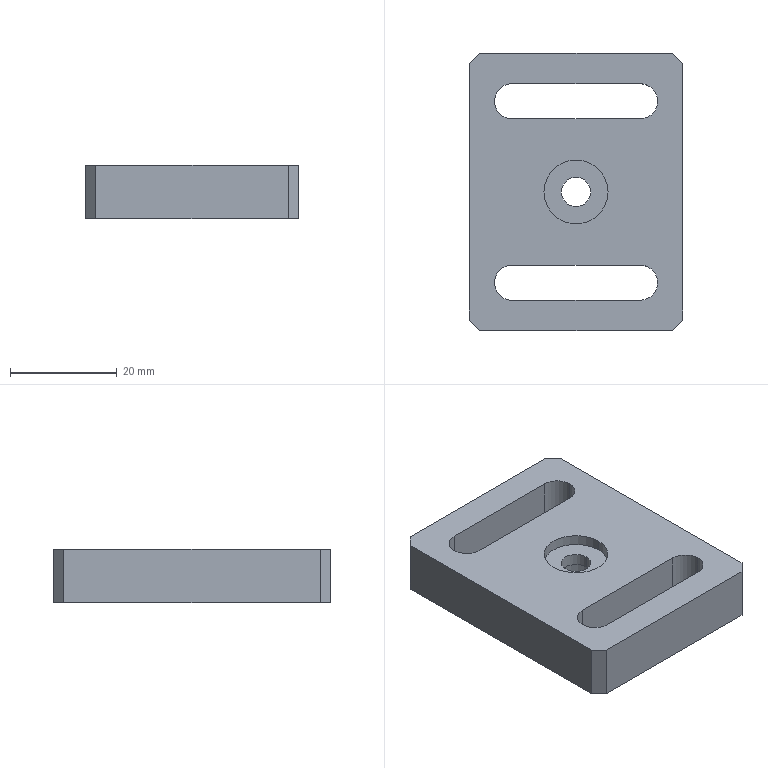Part | STEP file | 11-SMQ-00111 | 1 solid | 28 faces | box 40 x 52 x 10 mm | volume 16139 mm3 | plane 16 | cylinder 12 | commonest cylinder face diameters 6.6 x6 5.5 x2 10 x2 12 x2
STEP:
#1=CARTESIAN_POINT('',(15.3,-17.,0.));
#2=VERTEX_POINT('',#1);
#3=CARTESIAN_POINT('',(12.,-13.7,0.));
#4=VERTEX_POINT('',#3);
#5=CARTESIAN_POINT('',(12.,-17.,0.));
#6=DIRECTION('',(0.,0.,1.));
#7=DIRECTION('',(1.,0.,0.));
#8=AXIS2_PLACEMENT_3D('',#5,#6,#7);
#9=CIRCLE('',#8,3.3);
#10=EDGE_CURVE('',#2,#4,#9,.T.);
#11=ORIENTED_EDGE('',*,*,#10,.F.);
#12=CARTESIAN_POINT('',(15.3,-17.,10.));
#13=VERTEX_POINT('',#12);
#14=CARTESIAN_POINT('',(15.3,-17.,0.));
#15=DIRECTION('',(0.,0.,1.));
#16=VECTOR('',#15,1000.);
#17=LINE('',#14,#16);
#18=EDGE_CURVE('',#2,#13,#17,.T.);
#19=ORIENTED_EDGE('',*,*,#18,.T.);
#20=CARTESIAN_POINT('',(12.,-13.7,10.));
#21=VERTEX_POINT('',#20);
#22=CARTESIAN_POINT('',(12.,-17.,10.));
#23=DIRECTION('',(0.,0.,1.));
#24=DIRECTION('',(1.,0.,0.));
#25=AXIS2_PLACEMENT_3D('',#22,#23,#24);
#26=CIRCLE('',#25,3.3);
#27=EDGE_CURVE('',#13,#21,#26,.T.);
#28=ORIENTED_EDGE('',*,*,#27,.T.);
#29=CARTESIAN_POINT('',(12.,-13.7,0.));
#30=DIRECTION('',(0.,0.,1.));
#31=VECTOR('',#30,1000.);
#32=LINE('',#29,#31);
#33=EDGE_CURVE('',#4,#21,#32,.T.);
#34=ORIENTED_EDGE('',*,*,#33,.F.);
#35=EDGE_LOOP('',(#11,#19,#28,#34));
#36=FACE_OUTER_BOUND('',#35,.T.);
#37=CARTESIAN_POINT('',(12.,-17.,0.));
#38=DIRECTION('',(0.,0.,1.));
#39=DIRECTION('',(1.,0.,0.));
#40=AXIS2_PLACEMENT_3D('',#37,#38,#39);
#41=CYLINDRICAL_SURFACE('',#40,3.3);
#42=ADVANCED_FACE('',(#36),#41,.F.);
#43=CARTESIAN_POINT('',(15.3,17.,0.));
#44=VERTEX_POINT('',#43);
#45=CARTESIAN_POINT('',(12.,20.3,0.));
#46=VERTEX_POINT('',#45);
#47=CARTESIAN_POINT('',(12.,17.,0.));
#48=DIRECTION('',(0.,0.,1.));
#49=DIRECTION('',(1.,0.,0.));
#50=AXIS2_PLACEMENT_3D('',#47,#48,#49);
#51=CIRCLE('',#50,3.3);
#52=EDGE_CURVE('',#44,#46,#51,.T.);
#53=ORIENTED_EDGE('',*,*,#52,.F.);
#54=CARTESIAN_POINT('',(15.3,17.,10.));
#55=VERTEX_POINT('',#54);
#56=CARTESIAN_POINT('',(15.3,17.,0.));
#57=DIRECTION('',(0.,0.,1.));
#58=VECTOR('',#57,1000.);
#59=LINE('',#56,#58);
#60=EDGE_CURVE('',#44,#55,#59,.T.);
#61=ORIENTED_EDGE('',*,*,#60,.T.);
#62=CARTESIAN_POINT('',(12.,20.3,10.));
#63=VERTEX_POINT('',#62);
#64=CARTESIAN_POINT('',(12.,17.,10.));
#65=DIRECTION('',(0.,0.,1.));
#66=DIRECTION('',(1.,0.,0.));
#67=AXIS2_PLACEMENT_3D('',#64,#65,#66);
#68=CIRCLE('',#67,3.3);
#69=EDGE_CURVE('',#55,#63,#68,.T.);
#70=ORIENTED_EDGE('',*,*,#69,.T.);
#71=CARTESIAN_POINT('',(12.,20.3,0.));
#72=DIRECTION('',(0.,0.,1.));
#73=VECTOR('',#72,1000.);
#74=LINE('',#71,#73);
#75=EDGE_CURVE('',#46,#63,#74,.T.);
#76=ORIENTED_EDGE('',*,*,#75,.F.);
#77=EDGE_LOOP('',(#53,#61,#70,#76));
#78=FACE_OUTER_BOUND('',#77,.T.);
#79=CARTESIAN_POINT('',(12.,17.,0.));
#80=DIRECTION('',(0.,0.,1.));
#81=DIRECTION('',(1.,0.,0.));
#82=AXIS2_PLACEMENT_3D('',#79,#80,#81);
#83=CYLINDRICAL_SURFACE('',#82,3.3);
#84=ADVANCED_FACE('',(#78),#83,.F.);
#85=CARTESIAN_POINT('',(5.,0.,5.7));
#86=VERTEX_POINT('',#85);
#87=CARTESIAN_POINT('',(-5.,0.,5.7));
#88=VERTEX_POINT('',#87);
#89=CARTESIAN_POINT('',(0.,0.,5.7));
#90=DIRECTION('',(0.,0.,-1.));
#91=DIRECTION('',(-1.,0.,0.));
#92=AXIS2_PLACEMENT_3D('',#89,#90,#91);
#93=CIRCLE('',#92,5.);
#94=EDGE_CURVE('',#86,#88,#93,.T.);
#95=ORIENTED_EDGE('',*,*,#94,.F.);
#96=CARTESIAN_POINT('',(5.,0.,0.));
#97=VERTEX_POINT('',#96);
#98=CARTESIAN_POINT('',(5.,0.,0.));
#99=DIRECTION('',(0.,0.,-1.));
#100=VECTOR('',#99,1000.);
#101=LINE('',#98,#100);
#102=EDGE_CURVE('',#86,#97,#101,.T.);
#103=ORIENTED_EDGE('',*,*,#102,.T.);
#104=CARTESIAN_POINT('',(-5.,0.,0.));
#105=VERTEX_POINT('',#104);
#106=CARTESIAN_POINT('',(0.,0.,0.));
#107=DIRECTION('',(0.,0.,-1.));
#108=DIRECTION('',(-1.,0.,0.));
#109=AXIS2_PLACEMENT_3D('',#106,#107,#108);
#110=CIRCLE('',#109,5.);
#111=EDGE_CURVE('',#97,#105,#110,.T.);
#112=ORIENTED_EDGE('',*,*,#111,.T.);
#113=CARTESIAN_POINT('',(-5.,0.,0.));
#114=DIRECTION('',(0.,0.,-1.));
#115=VECTOR('',#114,1000.);
#116=LINE('',#113,#115);
#117=EDGE_CURVE('',#88,#105,#116,.T.);
#118=ORIENTED_EDGE('',*,*,#117,.F.);
#119=EDGE_LOOP('',(#95,#103,#112,#118));
#120=FACE_OUTER_BOUND('',#119,.T.);
#121=CARTESIAN_POINT('',(0.,0.,0.));
#122=DIRECTION('',(0.,0.,-1.));
#123=DIRECTION('',(-1.,0.,0.));
#124=AXIS2_PLACEMENT_3D('',#121,#122,#123);
#125=CYLINDRICAL_SURFACE('',#124,5.);
#126=ADVANCED_FACE('',(#120),#125,.F.);
#127=CARTESIAN_POINT('',(-2.75,0.,8.));
#128=VERTEX_POINT('',#127);
#129=CARTESIAN_POINT('',(2.75,0.,8.));
#130=VERTEX_POINT('',#129);
#131=CARTESIAN_POINT('',(0.,0.,8.));
#132=DIRECTION('',(0.,0.,1.));
#133=DIRECTION('',(1.,0.,0.));
#134=AXIS2_PLACEMENT_3D('',#131,#132,#133);
#135=CIRCLE('',#134,2.75);
#136=EDGE_CURVE('',#128,#130,#135,.T.);
#137=ORIENTED_EDGE('',*,*,#136,.T.);
#138=CARTESIAN_POINT('',(2.75,0.,5.7));
#139=VERTEX_POINT('',#138);
#140=CARTESIAN_POINT('',(2.75,0.,0.));
#141=DIRECTION('',(0.,0.,-1.));
#142=VECTOR('',#141,1000.);
#143=LINE('',#140,#142);
#144=EDGE_CURVE('',#130,#139,#143,.T.);
#145=ORIENTED_EDGE('',*,*,#144,.T.);
#146=CARTESIAN_POINT('',(-2.75,0.,5.7));
#147=VERTEX_POINT('',#146);
#148=CARTESIAN_POINT('',(0.,0.,5.7));
#149=DIRECTION('',(0.,0.,-1.));
#150=DIRECTION('',(-1.,0.,0.));
#151=AXIS2_PLACEMENT_3D('',#148,#149,#150);
#152=CIRCLE('',#151,2.75);
#153=EDGE_CURVE('',#139,#147,#152,.T.);
#154=ORIENTED_EDGE('',*,*,#153,.T.);
#155=CARTESIAN_POINT('',(-2.75,0.,0.));
#156=DIRECTION('',(0.,0.,-1.));
#157=VECTOR('',#156,1000.);
#158=LINE('',#155,#157);
#159=EDGE_CURVE('',#128,#147,#158,.T.);
#160=ORIENTED_EDGE('',*,*,#159,.F.);
#161=EDGE_LOOP('',(#137,#145,#154,#160));
#162=FACE_OUTER_BOUND('',#161,.T.);
#163=CARTESIAN_POINT('',(0.,0.,0.));
#164=DIRECTION('',(0.,0.,-1.));
#165=DIRECTION('',(-1.,0.,0.));
#166=AXIS2_PLACEMENT_3D('',#163,#164,#165);
#167=CYLINDRICAL_SURFACE('',#166,2.75);
#168=ADVANCED_FACE('',(#162),#167,.F.);
#169=CARTESIAN_POINT('',(-6.,0.,8.));
#170=VERTEX_POINT('',#169);
#171=CARTESIAN_POINT('',(6.,0.,8.));
#172=VERTEX_POINT('',#171);
#173=CARTESIAN_POINT('',(0.,0.,8.));
#174=DIRECTION('',(0.,0.,1.));
#175=DIRECTION('',(1.,0.,0.));
#176=AXIS2_PLACEMENT_3D('',#173,#174,#175);
#177=CIRCLE('',#176,6.);
#178=EDGE_CURVE('',#170,#172,#177,.T.);
#179=ORIENTED_EDGE('',*,*,#178,.F.);
#180=CARTESIAN_POINT('',(-6.,0.,10.));
#181=VERTEX_POINT('',#180);
#182=CARTESIAN_POINT('',(-6.,0.,8.));
#183=DIRECTION('',(0.,0.,1.));
#184=VECTOR('',#183,1000.);
#185=LINE('',#182,#184);
#186=EDGE_CURVE('',#170,#181,#185,.T.);
#187=ORIENTED_EDGE('',*,*,#186,.T.);
#188=CARTESIAN_POINT('',(6.,0.,10.));
#189=VERTEX_POINT('',#188);
#190=CARTESIAN_POINT('',(0.,0.,10.));
#191=DIRECTION('',(0.,0.,1.));
#192=DIRECTION('',(1.,0.,0.));
#193=AXIS2_PLACEMENT_3D('',#190,#191,#192);
#194=CIRCLE('',#193,6.);
#195=EDGE_CURVE('',#181,#189,#194,.T.);
#196=ORIENTED_EDGE('',*,*,#195,.T.);
#197=CARTESIAN_POINT('',(6.,0.,8.));
#198=DIRECTION('',(0.,0.,1.));
#199=VECTOR('',#198,1000.);
#200=LINE('',#197,#199);
#201=EDGE_CURVE('',#172,#189,#200,.T.);
#202=ORIENTED_EDGE('',*,*,#201,.F.);
#203=EDGE_LOOP('',(#179,#187,#196,#202));
#204=FACE_OUTER_BOUND('',#203,.T.);
#205=CARTESIAN_POINT('',(0.,0.,8.));
#206=DIRECTION('',(0.,0.,1.));
#207=DIRECTION('',(1.,0.,0.));
#208=AXIS2_PLACEMENT_3D('',#205,#206,#207);
#209=CYLINDRICAL_SURFACE('',#208,6.);
#210=ADVANCED_FACE('',(#204),#209,.F.);
#211=CARTESIAN_POINT('',(20.,-24.,10.));
#212=VERTEX_POINT('',#211);
#213=CARTESIAN_POINT('',(20.,24.,10.));
#214=VERTEX_POINT('',#213);
#215=CARTESIAN_POINT('',(20.,-26.,10.));
#216=DIRECTION('',(0.,1.,0.));
#217=VECTOR('',#216,1000.);
#218=LINE('',#215,#217);
#219=EDGE_CURVE('',#212,#214,#218,.T.);
#220=ORIENTED_EDGE('',*,*,#219,.F.);
#221=CARTESIAN_POINT('',(20.,-24.,0.));
#222=VERTEX_POINT('',#221);
#223=CARTESIAN_POINT('',(20.,-24.,10.));
#224=DIRECTION('',(0.,0.,-1.));
#225=VECTOR('',#224,1000.);
#226=LINE('',#223,#225);
#227=EDGE_CURVE('',#212,#222,#226,.T.);
#228=ORIENTED_EDGE('',*,*,#227,.T.);
#229=CARTESIAN_POINT('',(20.,24.,0.));
#230=VERTEX_POINT('',#229);
#231=CARTESIAN_POINT('',(20.,-26.,0.));
#232=DIRECTION('',(0.,1.,0.));
#233=VECTOR('',#232,1000.);
#234=LINE('',#231,#233);
#235=EDGE_CURVE('',#222,#230,#234,.T.);
#236=ORIENTED_EDGE('',*,*,#235,.T.);
#237=CARTESIAN_POINT('',(20.,24.,10.));
#238=DIRECTION('',(0.,0.,1.));
#239=VECTOR('',#238,1000.);
#240=LINE('',#237,#239);
#241=EDGE_CURVE('',#230,#214,#240,.T.);
#242=ORIENTED_EDGE('',*,*,#241,.T.);
#243=EDGE_LOOP('',(#220,#228,#236,#242));
#244=FACE_OUTER_BOUND('',#243,.T.);
#245=CARTESIAN_POINT('',(20.,-26.,10.));
#246=DIRECTION('',(-1.,0.,0.));
#247=DIRECTION('',(0.,0.,1.));
#248=AXIS2_PLACEMENT_3D('',#245,#246,#247);
#249=PLANE('',#248);
#250=ADVANCED_FACE('',(#244),#249,.F.);
#251=CARTESIAN_POINT('',(18.,26.,10.));
#252=VERTEX_POINT('',#251);
#253=CARTESIAN_POINT('',(-18.,26.,10.));
#254=VERTEX_POINT('',#253);
#255=CARTESIAN_POINT('',(-20.,26.,10.));
#256=DIRECTION('',(-1.,0.,0.));
#257=VECTOR('',#256,1000.);
#258=LINE('',#255,#257);
#259=EDGE_CURVE('',#252,#254,#258,.T.);
#260=ORIENTED_EDGE('',*,*,#259,.F.);
#261=CARTESIAN_POINT('',(18.,26.,0.));
#262=VERTEX_POINT('',#261);
#263=CARTESIAN_POINT('',(18.,26.,10.));
#264=DIRECTION('',(0.,0.,-1.));
#265=VECTOR('',#264,1000.);
#266=LINE('',#263,#265);
#267=EDGE_CURVE('',#252,#262,#266,.T.);
#268=ORIENTED_EDGE('',*,*,#267,.T.);
#269=CARTESIAN_POINT('',(-18.,26.,0.));
#270=VERTEX_POINT('',#269);
#271=CARTESIAN_POINT('',(-20.,26.,0.));
#272=DIRECTION('',(-1.,0.,0.));
#273=VECTOR('',#272,1000.);
#274=LINE('',#271,#273);
#275=EDGE_CURVE('',#262,#270,#274,.T.);
#276=ORIENTED_EDGE('',*,*,#275,.T.);
#277=CARTESIAN_POINT('',(-18.,26.,10.));
#278=DIRECTION('',(0.,0.,1.));
#279=VECTOR('',#278,1000.);
#280=LINE('',#277,#279);
#281=EDGE_CURVE('',#270,#254,#280,.T.);
#282=ORIENTED_EDGE('',*,*,#281,.T.);
#283=EDGE_LOOP('',(#260,#268,#276,#282));
#284=FACE_OUTER_BOUND('',#283,.T.);
#285=CARTESIAN_POINT('',(-20.,26.,10.));
#286=DIRECTION('',(0.,-1.,0.));
#287=DIRECTION('',(0.,0.,-1.));
#288=AXIS2_PLACEMENT_3D('',#285,#286,#287);
#289=PLANE('',#288);
#290=ADVANCED_FACE('',(#284),#289,.F.);
#291=CARTESIAN_POINT('',(-20.,24.,0.));
#292=VERTEX_POINT('',#291);
#293=CARTESIAN_POINT('',(-20.,-24.,0.));
#294=VERTEX_POINT('',#293);
#295=CARTESIAN_POINT('',(-20.,-26.,0.));
#296=DIRECTION('',(0.,-1.,0.));
#297=VECTOR('',#296,1000.);
#298=LINE('',#295,#297);
#299=EDGE_CURVE('',#292,#294,#298,.T.);
#300=ORIENTED_EDGE('',*,*,#299,.T.);
#301=CARTESIAN_POINT('',(-20.,-24.,10.));
#302=VERTEX_POINT('',#301);
#303=CARTESIAN_POINT('',(-20.,-24.,10.));
#304=DIRECTION('',(0.,0.,1.));
#305=VECTOR('',#304,1000.);
#306=LINE('',#303,#305);
#307=EDGE_CURVE('',#294,#302,#306,.T.);
#308=ORIENTED_EDGE('',*,*,#307,.T.);
#309=CARTESIAN_POINT('',(-20.,24.,10.));
#310=VERTEX_POINT('',#309);
#311=CARTESIAN_POINT('',(-20.,-26.,10.));
#312=DIRECTION('',(0.,-1.,0.));
#313=VECTOR('',#312,1000.);
#314=LINE('',#311,#313);
#315=EDGE_CURVE('',#310,#302,#314,.T.);
#316=ORIENTED_EDGE('',*,*,#315,.F.);
#317=CARTESIAN_POINT('',(-20.,24.,10.));
#318=DIRECTION('',(0.,0.,-1.));
#319=VECTOR('',#318,1000.);
#320=LINE('',#317,#319);
#321=EDGE_CURVE('',#310,#292,#320,.T.);
#322=ORIENTED_EDGE('',*,*,#321,.T.);
#323=EDGE_LOOP('',(#300,#308,#316,#322));
#324=FACE_OUTER_BOUND('',#323,.T.);
#325=CARTESIAN_POINT('',(-20.,-26.,10.));
#326=DIRECTION('',(1.,0.,0.));
#327=DIRECTION('',(0.,0.,-1.));
#328=AXIS2_PLACEMENT_3D('',#325,#326,#327);
#329=PLANE('',#328);
#330=ADVANCED_FACE('',(#324),#329,.F.);
#331=CARTESIAN_POINT('',(-18.,-26.,0.));
#332=VERTEX_POINT('',#331);
#333=CARTESIAN_POINT('',(18.,-26.,0.));
#334=VERTEX_POINT('',#333);
#335=CARTESIAN_POINT('',(-20.,-26.,0.));
#336=DIRECTION('',(1.,0.,0.));
#337=VECTOR('',#336,1000.);
#338=LINE('',#335,#337);
#339=EDGE_CURVE('',#332,#334,#338,.T.);
#340=ORIENTED_EDGE('',*,*,#339,.T.);
#341=CARTESIAN_POINT('',(18.,-26.,10.));
#342=VERTEX_POINT('',#341);
#343=CARTESIAN_POINT('',(18.,-26.,10.));
#344=DIRECTION('',(0.,0.,1.));
#345=VECTOR('',#344,1000.);
#346=LINE('',#343,#345);
#347=EDGE_CURVE('',#334,#342,#346,.T.);
#348=ORIENTED_EDGE('',*,*,#347,.T.);
#349=CARTESIAN_POINT('',(-18.,-26.,10.));
#350=VERTEX_POINT('',#349);
#351=CARTESIAN_POINT('',(-20.,-26.,10.));
#352=DIRECTION('',(1.,0.,0.));
#353=VECTOR('',#352,1000.);
#354=LINE('',#351,#353);
#355=EDGE_CURVE('',#350,#342,#354,.T.);
#356=ORIENTED_EDGE('',*,*,#355,.F.);
#357=CARTESIAN_POINT('',(-18.,-26.,10.));
#358=DIRECTION('',(0.,0.,-1.));
#359=VECTOR('',#358,1000.);
#360=LINE('',#357,#359);
#361=EDGE_CURVE('',#350,#332,#360,.T.);
#362=ORIENTED_EDGE('',*,*,#361,.T.);
#363=EDGE_LOOP('',(#340,#348,#356,#362));
#364=FACE_OUTER_BOUND('',#363,.T.);
#365=CARTESIAN_POINT('',(-20.,-26.,10.));
#366=DIRECTION('',(0.,1.,0.));
#367=DIRECTION('',(0.,0.,1.));
#368=AXIS2_PLACEMENT_3D('',#365,#366,#367);
#369=PLANE('',#368);
#370=ADVANCED_FACE('',(#364),#369,.F.);
#371=CARTESIAN_POINT('',(-12.,-13.7,10.));
#372=VERTEX_POINT('',#371);
#373=CARTESIAN_POINT('',(12.,-13.7,10.));
#374=DIRECTION('',(-1.,0.,0.));
#375=VECTOR('',#374,1000.);
#376=LINE('',#373,#375);
#377=EDGE_CURVE('',#21,#372,#376,.T.);
#378=ORIENTED_EDGE('',*,*,#377,.F.);
#379=ORIENTED_EDGE('',*,*,#27,.F.);
#380=CARTESIAN_POINT('',(12.,-20.3,10.));
#381=VERTEX_POINT('',#380);
#382=CARTESIAN_POINT('',(12.,-17.,10.));
#383=DIRECTION('',(0.,0.,1.));
#384=DIRECTION('',(1.,0.,0.));
#385=AXIS2_PLACEMENT_3D('',#382,#383,#384);
#386=CIRCLE('',#385,3.3);
#387=EDGE_CURVE('',#381,#13,#386,.T.);
#388=ORIENTED_EDGE('',*,*,#387,.F.);
#389=CARTESIAN_POINT('',(-12.,-20.3,10.));
#390=VERTEX_POINT('',#389);
#391=CARTESIAN_POINT('',(12.,-20.3,10.));
#392=DIRECTION('',(1.,0.,0.));
#393=VECTOR('',#392,1000.);
#394=LINE('',#391,#393);
#395=EDGE_CURVE('',#390,#381,#394,.T.);
#396=ORIENTED_EDGE('',*,*,#395,.F.);
#397=CARTESIAN_POINT('',(-12.,-17.,10.));
#398=DIRECTION('',(0.,0.,1.));
#399=DIRECTION('',(1.,0.,0.));
#400=AXIS2_PLACEMENT_3D('',#397,#398,#399);
#401=CIRCLE('',#400,3.3);
#402=EDGE_CURVE('',#372,#390,#401,.T.);
#403=ORIENTED_EDGE('',*,*,#402,.F.);
#404=EDGE_LOOP('',(#378,#379,#388,#396,#403));
#405=FACE_BOUND('',#404,.T.);
#406=CARTESIAN_POINT('',(-12.,20.3,10.));
#407=VERTEX_POINT('',#406);
#408=CARTESIAN_POINT('',(12.,20.3,10.));
#409=DIRECTION('',(-1.,0.,0.));
#410=VECTOR('',#409,1000.);
#411=LINE('',#408,#410);
#412=EDGE_CURVE('',#63,#407,#411,.T.);
#413=ORIENTED_EDGE('',*,*,#412,.F.);
#414=ORIENTED_EDGE('',*,*,#69,.F.);
#415=CARTESIAN_POINT('',(12.,13.7,10.));
#416=VERTEX_POINT('',#415);
#417=CARTESIAN_POINT('',(12.,17.,10.));
#418=DIRECTION('',(0.,0.,1.));
#419=DIRECTION('',(1.,0.,0.));
#420=AXIS2_PLACEMENT_3D('',#417,#418,#419);
#421=CIRCLE('',#420,3.3);
#422=EDGE_CURVE('',#416,#55,#421,.T.);
#423=ORIENTED_EDGE('',*,*,#422,.F.);
#424=CARTESIAN_POINT('',(-12.,13.7,10.));
#425=VERTEX_POINT('',#424);
#426=CARTESIAN_POINT('',(12.,13.7,10.));
#427=DIRECTION('',(1.,0.,0.));
#428=VECTOR('',#427,1000.);
#429=LINE('',#426,#428);
#430=EDGE_CURVE('',#425,#416,#429,.T.);
#431=ORIENTED_EDGE('',*,*,#430,.F.);
#432=CARTESIAN_POINT('',(-12.,17.,10.));
#433=DIRECTION('',(0.,0.,1.));
#434=DIRECTION('',(1.,0.,0.));
#435=AXIS2_PLACEMENT_3D('',#432,#433,#434);
#436=CIRCLE('',#435,3.3);
#437=EDGE_CURVE('',#407,#425,#436,.T.);
#438=ORIENTED_EDGE('',*,*,#437,.F.);
#439=EDGE_LOOP('',(#413,#414,#423,#431,#438));
#440=FACE_BOUND('',#439,.T.);
#441=CARTESIAN_POINT('',(0.,0.,10.));
#442=DIRECTION('',(0.,0.,1.));
#443=DIRECTION('',(1.,0.,0.));
#444=AXIS2_PLACEMENT_3D('',#441,#442,#443);
#445=CIRCLE('',#444,6.);
#446=EDGE_CURVE('',#189,#181,#445,.T.);
#447=ORIENTED_EDGE('',*,*,#446,.F.);
#448=ORIENTED_EDGE('',*,*,#195,.F.);
#449=EDGE_LOOP('',(#447,#448));
#450=FACE_BOUND('',#449,.T.);
#451=ORIENTED_EDGE('',*,*,#355,.T.);
#452=CARTESIAN_POINT('',(20.,-24.,10.));
#453=DIRECTION('',(0.7071,0.7071,0.));
#454=VECTOR('',#453,1000.);
#455=LINE('',#452,#454);
#456=EDGE_CURVE('',#342,#212,#455,.T.);
#457=ORIENTED_EDGE('',*,*,#456,.T.);
#458=ORIENTED_EDGE('',*,*,#219,.T.);
#459=CARTESIAN_POINT('',(18.,26.,10.));
#460=DIRECTION('',(-0.7071,0.7071,0.));
#461=VECTOR('',#460,1000.);
#462=LINE('',#459,#461);
#463=EDGE_CURVE('',#214,#252,#462,.T.);
#464=ORIENTED_EDGE('',*,*,#463,.T.);
#465=ORIENTED_EDGE('',*,*,#259,.T.);
#466=CARTESIAN_POINT('',(-20.,24.,10.));
#467=DIRECTION('',(-0.7071,-0.7071,0.));
#468=VECTOR('',#467,1000.);
#469=LINE('',#466,#468);
#470=EDGE_CURVE('',#254,#310,#469,.T.);
#471=ORIENTED_EDGE('',*,*,#470,.T.);
#472=ORIENTED_EDGE('',*,*,#315,.T.);
#473=CARTESIAN_POINT('',(-18.,-26.,10.));
#474=DIRECTION('',(0.7071,-0.7071,0.));
#475=VECTOR('',#474,1000.);
#476=LINE('',#473,#475);
#477=EDGE_CURVE('',#302,#350,#476,.T.);
#478=ORIENTED_EDGE('',*,*,#477,.T.);
#479=EDGE_LOOP('',(#451,#457,#458,#464,#465,#471,#472,#478));
#480=FACE_OUTER_BOUND('',#479,.T.);
#481=CARTESIAN_POINT('',(0.,0.,10.));
#482=DIRECTION('',(0.,0.,-1.));
#483=DIRECTION('',(-1.,0.,0.));
#484=AXIS2_PLACEMENT_3D('',#481,#482,#483);
#485=PLANE('',#484);
#486=ADVANCED_FACE('',(#405,#440,#450,#480),#485,.F.);
#487=CARTESIAN_POINT('',(12.,-20.3,0.));
#488=VERTEX_POINT('',#487);
#489=CARTESIAN_POINT('',(12.,-17.,0.));
#490=DIRECTION('',(0.,0.,1.));
#491=DIRECTION('',(1.,0.,0.));
#492=AXIS2_PLACEMENT_3D('',#489,#490,#491);
#493=CIRCLE('',#492,3.3);
#494=EDGE_CURVE('',#488,#2,#493,.T.);
#495=ORIENTED_EDGE('',*,*,#494,.T.);
#496=ORIENTED_EDGE('',*,*,#10,.T.);
#497=CARTESIAN_POINT('',(-12.,-13.7,0.));
#498=VERTEX_POINT('',#497);
#499=CARTESIAN_POINT('',(12.,-13.7,0.));
#500=DIRECTION('',(-1.,0.,0.));
#501=VECTOR('',#500,1000.);
#502=LINE('',#499,#501);
#503=EDGE_CURVE('',#4,#498,#502,.T.);
#504=ORIENTED_EDGE('',*,*,#503,.T.);
#505=CARTESIAN_POINT('',(-12.,-20.3,0.));
#506=VERTEX_POINT('',#505);
#507=CARTESIAN_POINT('',(-12.,-17.,0.));
#508=DIRECTION('',(0.,0.,1.));
#509=DIRECTION('',(1.,0.,0.));
#510=AXIS2_PLACEMENT_3D('',#507,#508,#509);
#511=CIRCLE('',#510,3.3);
#512=EDGE_CURVE('',#498,#506,#511,.T.);
#513=ORIENTED_EDGE('',*,*,#512,.T.);
#514=CARTESIAN_POINT('',(12.,-20.3,0.));
#515=DIRECTION('',(1.,0.,0.));
#516=VECTOR('',#515,1000.);
#517=LINE('',#514,#516);
#518=EDGE_CURVE('',#506,#488,#517,.T.);
#519=ORIENTED_EDGE('',*,*,#518,.T.);
#520=EDGE_LOOP('',(#495,#496,#504,#513,#519));
#521=FACE_BOUND('',#520,.T.);
#522=CARTESIAN_POINT('',(12.,13.7,0.));
#523=VERTEX_POINT('',#522);
#524=CARTESIAN_POINT('',(12.,17.,0.));
#525=DIRECTION('',(0.,0.,1.));
#526=DIRECTION('',(1.,0.,0.));
#527=AXIS2_PLACEMENT_3D('',#524,#525,#526);
#528=CIRCLE('',#527,3.3);
#529=EDGE_CURVE('',#523,#44,#528,.T.);
#530=ORIENTED_EDGE('',*,*,#529,.T.);
#531=ORIENTED_EDGE('',*,*,#52,.T.);
#532=CARTESIAN_POINT('',(-12.,20.3,0.));
#533=VERTEX_POINT('',#532);
#534=CARTESIAN_POINT('',(12.,20.3,0.));
#535=DIRECTION('',(-1.,0.,0.));
#536=VECTOR('',#535,1000.);
#537=LINE('',#534,#536);
#538=EDGE_CURVE('',#46,#533,#537,.T.);
#539=ORIENTED_EDGE('',*,*,#538,.T.);
#540=CARTESIAN_POINT('',(-12.,13.7,0.));
#541=VERTEX_POINT('',#540);
#542=CARTESIAN_POINT('',(-12.,17.,0.));
#543=DIRECTION('',(0.,0.,1.));
#544=DIRECTION('',(1.,0.,0.));
#545=AXIS2_PLACEMENT_3D('',#542,#543,#544);
#546=CIRCLE('',#545,3.3);
#547=EDGE_CURVE('',#533,#541,#546,.T.);
#548=ORIENTED_EDGE('',*,*,#547,.T.);
#549=CARTESIAN_POINT('',(12.,13.7,0.));
#550=DIRECTION('',(1.,0.,0.));
#551=VECTOR('',#550,1000.);
#552=LINE('',#549,#551);
#553=EDGE_CURVE('',#541,#523,#552,.T.);
#554=ORIENTED_EDGE('',*,*,#553,.T.);
#555=EDGE_LOOP('',(#530,#531,#539,#548,#554));
#556=FACE_BOUND('',#555,.T.);
#557=CARTESIAN_POINT('',(0.,0.,0.));
#558=DIRECTION('',(0.,0.,-1.));
#559=DIRECTION('',(-1.,0.,0.));
#560=AXIS2_PLACEMENT_3D('',#557,#558,#559);
#561=CIRCLE('',#560,5.);
#562=EDGE_CURVE('',#105,#97,#561,.T.);
#563=ORIENTED_EDGE('',*,*,#562,.F.);
#564=ORIENTED_EDGE('',*,*,#111,.F.);
#565=EDGE_LOOP('',(#563,#564));
#566=FACE_BOUND('',#565,.T.);
#567=ORIENTED_EDGE('',*,*,#235,.F.);
#568=CARTESIAN_POINT('',(22.,-22.,0.));
#569=DIRECTION('',(-0.7071,-0.7071,0.));
#570=VECTOR('',#569,1000.);
#571=LINE('',#568,#570);
#572=EDGE_CURVE('',#222,#334,#571,.T.);
#573=ORIENTED_EDGE('',*,*,#572,.T.);
#574=ORIENTED_EDGE('',*,*,#339,.F.);
#575=CARTESIAN_POINT('',(-22.,-22.,0.));
#576=DIRECTION('',(-0.7071,0.7071,0.));
#577=VECTOR('',#576,1000.);
#578=LINE('',#575,#577);
#579=EDGE_CURVE('',#332,#294,#578,.T.);
#580=ORIENTED_EDGE('',*,*,#579,.T.);
#581=ORIENTED_EDGE('',*,*,#299,.F.);
#582=CARTESIAN_POINT('',(-22.,22.,0.));
#583=DIRECTION('',(0.7071,0.7071,0.));
#584=VECTOR('',#583,1000.);
#585=LINE('',#582,#584);
#586=EDGE_CURVE('',#292,#270,#585,.T.);
#587=ORIENTED_EDGE('',*,*,#586,.T.);
#588=ORIENTED_EDGE('',*,*,#275,.F.);
#589=CARTESIAN_POINT('',(22.,22.,0.));
#590=DIRECTION('',(0.7071,-0.7071,0.));
#591=VECTOR('',#590,1000.);
#592=LINE('',#589,#591);
#593=EDGE_CURVE('',#262,#230,#592,.T.);
#594=ORIENTED_EDGE('',*,*,#593,.T.);
#595=EDGE_LOOP('',(#567,#573,#574,#580,#581,#587,#588,#594));
#596=FACE_OUTER_BOUND('',#595,.T.);
#597=CARTESIAN_POINT('',(0.,0.,0.));
#598=DIRECTION('',(0.,0.,-1.));
#599=DIRECTION('',(-1.,0.,0.));
#600=AXIS2_PLACEMENT_3D('',#597,#598,#599);
#601=PLANE('',#600);
#602=ADVANCED_FACE('',(#521,#556,#566,#596),#601,.T.);
#603=ORIENTED_EDGE('',*,*,#456,.F.);
#604=ORIENTED_EDGE('',*,*,#347,.F.);
#605=ORIENTED_EDGE('',*,*,#572,.F.);
#606=ORIENTED_EDGE('',*,*,#227,.F.);
#607=EDGE_LOOP('',(#603,#604,#605,#606));
#608=FACE_OUTER_BOUND('',#607,.T.);
#609=CARTESIAN_POINT('',(20.,-24.,10.));
#610=DIRECTION('',(-0.7071,0.7071,0.));
#611=DIRECTION('',(0.,0.,-1.));
#612=AXIS2_PLACEMENT_3D('',#609,#610,#611);
#613=PLANE('',#612);
#614=ADVANCED_FACE('',(#608),#613,.F.);
#615=ORIENTED_EDGE('',*,*,#463,.F.);
#616=ORIENTED_EDGE('',*,*,#241,.F.);
#617=ORIENTED_EDGE('',*,*,#593,.F.);
#618=ORIENTED_EDGE('',*,*,#267,.F.);
#619=EDGE_LOOP('',(#615,#616,#617,#618));
#620=FACE_OUTER_BOUND('',#619,.T.);
#621=CARTESIAN_POINT('',(18.,26.,10.));
#622=DIRECTION('',(-0.7071,-0.7071,0.));
#623=DIRECTION('',(0.,0.,-1.));
#624=AXIS2_PLACEMENT_3D('',#621,#622,#623);
#625=PLANE('',#624);
#626=ADVANCED_FACE('',(#620),#625,.F.);
#627=ORIENTED_EDGE('',*,*,#477,.F.);
#628=ORIENTED_EDGE('',*,*,#307,.F.);
#629=ORIENTED_EDGE('',*,*,#579,.F.);
#630=ORIENTED_EDGE('',*,*,#361,.F.);
#631=EDGE_LOOP('',(#627,#628,#629,#630));
#632=FACE_OUTER_BOUND('',#631,.T.);
#633=CARTESIAN_POINT('',(-18.,-26.,10.));
#634=DIRECTION('',(0.7071,0.7071,0.));
#635=DIRECTION('',(0.,0.,-1.));
#636=AXIS2_PLACEMENT_3D('',#633,#634,#635);
#637=PLANE('',#636);
#638=ADVANCED_FACE('',(#632),#637,.F.);
#639=ORIENTED_EDGE('',*,*,#470,.F.);
#640=ORIENTED_EDGE('',*,*,#281,.F.);
#641=ORIENTED_EDGE('',*,*,#586,.F.);
#642=ORIENTED_EDGE('',*,*,#321,.F.);
#643=EDGE_LOOP('',(#639,#640,#641,#642));
#644=FACE_OUTER_BOUND('',#643,.T.);
#645=CARTESIAN_POINT('',(-20.,24.,10.));
#646=DIRECTION('',(0.7071,-0.7071,0.));
#647=DIRECTION('',(0.,0.,-1.));
#648=AXIS2_PLACEMENT_3D('',#645,#646,#647);
#649=PLANE('',#648);
#650=ADVANCED_FACE('',(#644),#649,.F.);
#651=ORIENTED_EDGE('',*,*,#186,.F.);
#652=CARTESIAN_POINT('',(0.,0.,8.));
#653=DIRECTION('',(0.,0.,1.));
#654=DIRECTION('',(1.,0.,0.));
#655=AXIS2_PLACEMENT_3D('',#652,#653,#654);
#656=CIRCLE('',#655,6.);
#657=EDGE_CURVE('',#172,#170,#656,.T.);
#658=ORIENTED_EDGE('',*,*,#657,.F.);
#659=ORIENTED_EDGE('',*,*,#201,.T.);
#660=ORIENTED_EDGE('',*,*,#446,.T.);
#661=EDGE_LOOP('',(#651,#658,#659,#660));
#662=FACE_OUTER_BOUND('',#661,.T.);
#663=CARTESIAN_POINT('',(0.,0.,8.));
#664=DIRECTION('',(0.,0.,1.));
#665=DIRECTION('',(1.,0.,0.));
#666=AXIS2_PLACEMENT_3D('',#663,#664,#665);
#667=CYLINDRICAL_SURFACE('',#666,6.);
#668=ADVANCED_FACE('',(#662),#667,.F.);
#669=ORIENTED_EDGE('',*,*,#136,.F.);
#670=CARTESIAN_POINT('',(0.,0.,8.));
#671=DIRECTION('',(0.,0.,1.));
#672=DIRECTION('',(1.,0.,0.));
#673=AXIS2_PLACEMENT_3D('',#670,#671,#672);
#674=CIRCLE('',#673,2.75);
#675=EDGE_CURVE('',#130,#128,#674,.T.);
#676=ORIENTED_EDGE('',*,*,#675,.F.);
#677=EDGE_LOOP('',(#669,#676));
#678=FACE_BOUND('',#677,.T.);
#679=ORIENTED_EDGE('',*,*,#657,.T.);
#680=ORIENTED_EDGE('',*,*,#178,.T.);
#681=EDGE_LOOP('',(#679,#680));
#682=FACE_OUTER_BOUND('',#681,.T.);
#683=CARTESIAN_POINT('',(0.,0.,8.));
#684=DIRECTION('',(0.,0.,1.));
#685=DIRECTION('',(1.,0.,0.));
#686=AXIS2_PLACEMENT_3D('',#683,#684,#685);
#687=PLANE('',#686);
#688=ADVANCED_FACE('',(#678,#682),#687,.T.);
#689=ORIENTED_EDGE('',*,*,#144,.F.);
#690=ORIENTED_EDGE('',*,*,#675,.T.);
#691=ORIENTED_EDGE('',*,*,#159,.T.);
#692=CARTESIAN_POINT('',(0.,0.,5.7));
#693=DIRECTION('',(0.,0.,-1.));
#694=DIRECTION('',(-1.,0.,0.));
#695=AXIS2_PLACEMENT_3D('',#692,#693,#694);
#696=CIRCLE('',#695,2.75);
#697=EDGE_CURVE('',#147,#139,#696,.T.);
#698=ORIENTED_EDGE('',*,*,#697,.T.);
#699=EDGE_LOOP('',(#689,#690,#691,#698));
#700=FACE_OUTER_BOUND('',#699,.T.);
#701=CARTESIAN_POINT('',(0.,0.,0.));
#702=DIRECTION('',(0.,0.,-1.));
#703=DIRECTION('',(-1.,0.,0.));
#704=AXIS2_PLACEMENT_3D('',#701,#702,#703);
#705=CYLINDRICAL_SURFACE('',#704,2.75);
#706=ADVANCED_FACE('',(#700),#705,.F.);
#707=ORIENTED_EDGE('',*,*,#697,.F.);
#708=ORIENTED_EDGE('',*,*,#153,.F.);
#709=EDGE_LOOP('',(#707,#708));
#710=FACE_BOUND('',#709,.T.);
#711=CARTESIAN_POINT('',(0.,0.,5.7));
#712=DIRECTION('',(0.,0.,-1.));
#713=DIRECTION('',(-1.,0.,0.));
#714=AXIS2_PLACEMENT_3D('',#711,#712,#713);
#715=CIRCLE('',#714,5.);
#716=EDGE_CURVE('',#88,#86,#715,.T.);
#717=ORIENTED_EDGE('',*,*,#716,.T.);
#718=ORIENTED_EDGE('',*,*,#94,.T.);
#719=EDGE_LOOP('',(#717,#718));
#720=FACE_OUTER_BOUND('',#719,.T.);
#721=CARTESIAN_POINT('',(2.75,0.,5.7));
#722=DIRECTION('',(0.,0.,1.));
#723=DIRECTION('',(1.,0.,0.));
#724=AXIS2_PLACEMENT_3D('',#721,#722,#723);
#725=PLANE('',#724);
#726=ADVANCED_FACE('',(#710,#720),#725,.F.);
#727=ORIENTED_EDGE('',*,*,#102,.F.);
#728=ORIENTED_EDGE('',*,*,#716,.F.);
#729=ORIENTED_EDGE('',*,*,#117,.T.);
#730=ORIENTED_EDGE('',*,*,#562,.T.);
#731=EDGE_LOOP('',(#727,#728,#729,#730));
#732=FACE_OUTER_BOUND('',#731,.T.);
#733=CARTESIAN_POINT('',(0.,0.,0.));
#734=DIRECTION('',(0.,0.,-1.));
#735=DIRECTION('',(-1.,0.,0.));
#736=AXIS2_PLACEMENT_3D('',#733,#734,#735);
#737=CYLINDRICAL_SURFACE('',#736,5.);
#738=ADVANCED_FACE('',(#732),#737,.F.);
#739=ORIENTED_EDGE('',*,*,#60,.F.);
#740=ORIENTED_EDGE('',*,*,#529,.F.);
#741=CARTESIAN_POINT('',(12.,13.7,0.));
#742=DIRECTION('',(0.,0.,1.));
#743=VECTOR('',#742,1000.);
#744=LINE('',#741,#743);
#745=EDGE_CURVE('',#523,#416,#744,.T.);
#746=ORIENTED_EDGE('',*,*,#745,.T.);
#747=ORIENTED_EDGE('',*,*,#422,.T.);
#748=EDGE_LOOP('',(#739,#740,#746,#747));
#749=FACE_OUTER_BOUND('',#748,.T.);
#750=CARTESIAN_POINT('',(12.,17.,0.));
#751=DIRECTION('',(0.,0.,1.));
#752=DIRECTION('',(1.,0.,0.));
#753=AXIS2_PLACEMENT_3D('',#750,#751,#752);
#754=CYLINDRICAL_SURFACE('',#753,3.3);
#755=ADVANCED_FACE('',(#749),#754,.F.);
#756=ORIENTED_EDGE('',*,*,#430,.T.);
#757=ORIENTED_EDGE('',*,*,#745,.F.);
#758=ORIENTED_EDGE('',*,*,#553,.F.);
#759=CARTESIAN_POINT('',(-12.,13.7,0.));
#760=DIRECTION('',(0.,0.,1.));
#761=VECTOR('',#760,1000.);
#762=LINE('',#759,#761);
#763=EDGE_CURVE('',#541,#425,#762,.T.);
#764=ORIENTED_EDGE('',*,*,#763,.T.);
#765=EDGE_LOOP('',(#756,#757,#758,#764));
#766=FACE_OUTER_BOUND('',#765,.T.);
#767=CARTESIAN_POINT('',(12.,13.7,0.));
#768=DIRECTION('',(0.,-1.,0.));
#769=DIRECTION('',(0.,0.,-1.));
#770=AXIS2_PLACEMENT_3D('',#767,#768,#769);
#771=PLANE('',#770);
#772=ADVANCED_FACE('',(#766),#771,.F.);
#773=ORIENTED_EDGE('',*,*,#437,.T.);
#774=ORIENTED_EDGE('',*,*,#763,.F.);
#775=ORIENTED_EDGE('',*,*,#547,.F.);
#776=CARTESIAN_POINT('',(-12.,20.3,0.));
#777=DIRECTION('',(0.,0.,1.));
#778=VECTOR('',#777,1000.);
#779=LINE('',#776,#778);
#780=EDGE_CURVE('',#533,#407,#779,.T.);
#781=ORIENTED_EDGE('',*,*,#780,.T.);
#782=EDGE_LOOP('',(#773,#774,#775,#781));
#783=FACE_OUTER_BOUND('',#782,.T.);
#784=CARTESIAN_POINT('',(-12.,17.,0.));
#785=DIRECTION('',(0.,0.,1.));
#786=DIRECTION('',(1.,0.,0.));
#787=AXIS2_PLACEMENT_3D('',#784,#785,#786);
#788=CYLINDRICAL_SURFACE('',#787,3.3);
#789=ADVANCED_FACE('',(#783),#788,.F.);
#790=ORIENTED_EDGE('',*,*,#412,.T.);
#791=ORIENTED_EDGE('',*,*,#780,.F.);
#792=ORIENTED_EDGE('',*,*,#538,.F.);
#793=ORIENTED_EDGE('',*,*,#75,.T.);
#794=EDGE_LOOP('',(#790,#791,#792,#793));
#795=FACE_OUTER_BOUND('',#794,.T.);
#796=CARTESIAN_POINT('',(12.,20.3,0.));
#797=DIRECTION('',(0.,1.,0.));
#798=DIRECTION('',(0.,0.,1.));
#799=AXIS2_PLACEMENT_3D('',#796,#797,#798);
#800=PLANE('',#799);
#801=ADVANCED_FACE('',(#795),#800,.F.);
#802=ORIENTED_EDGE('',*,*,#18,.F.);
#803=ORIENTED_EDGE('',*,*,#494,.F.);
#804=CARTESIAN_POINT('',(12.,-20.3,0.));
#805=DIRECTION('',(0.,0.,1.));
#806=VECTOR('',#805,1000.);
#807=LINE('',#804,#806);
#808=EDGE_CURVE('',#488,#381,#807,.T.);
#809=ORIENTED_EDGE('',*,*,#808,.T.);
#810=ORIENTED_EDGE('',*,*,#387,.T.);
#811=EDGE_LOOP('',(#802,#803,#809,#810));
#812=FACE_OUTER_BOUND('',#811,.T.);
#813=CARTESIAN_POINT('',(12.,-17.,0.));
#814=DIRECTION('',(0.,0.,1.));
#815=DIRECTION('',(1.,0.,0.));
#816=AXIS2_PLACEMENT_3D('',#813,#814,#815);
#817=CYLINDRICAL_SURFACE('',#816,3.3);
#818=ADVANCED_FACE('',(#812),#817,.F.);
#819=ORIENTED_EDGE('',*,*,#395,.T.);
#820=ORIENTED_EDGE('',*,*,#808,.F.);
#821=ORIENTED_EDGE('',*,*,#518,.F.);
#822=CARTESIAN_POINT('',(-12.,-20.3,0.));
#823=DIRECTION('',(0.,0.,1.));
#824=VECTOR('',#823,1000.);
#825=LINE('',#822,#824);
#826=EDGE_CURVE('',#506,#390,#825,.T.);
#827=ORIENTED_EDGE('',*,*,#826,.T.);
#828=EDGE_LOOP('',(#819,#820,#821,#827));
#829=FACE_OUTER_BOUND('',#828,.T.);
#830=CARTESIAN_POINT('',(12.,-20.3,0.));
#831=DIRECTION('',(0.,-1.,0.));
#832=DIRECTION('',(0.,0.,-1.));
#833=AXIS2_PLACEMENT_3D('',#830,#831,#832);
#834=PLANE('',#833);
#835=ADVANCED_FACE('',(#829),#834,.F.);
#836=ORIENTED_EDGE('',*,*,#402,.T.);
#837=ORIENTED_EDGE('',*,*,#826,.F.);
#838=ORIENTED_EDGE('',*,*,#512,.F.);
#839=CARTESIAN_POINT('',(-12.,-13.7,0.));
#840=DIRECTION('',(0.,0.,1.));
#841=VECTOR('',#840,1000.);
#842=LINE('',#839,#841);
#843=EDGE_CURVE('',#498,#372,#842,.T.);
#844=ORIENTED_EDGE('',*,*,#843,.T.);
#845=EDGE_LOOP('',(#836,#837,#838,#844));
#846=FACE_OUTER_BOUND('',#845,.T.);
#847=CARTESIAN_POINT('',(-12.,-17.,0.));
#848=DIRECTION('',(0.,0.,1.));
#849=DIRECTION('',(1.,0.,0.));
#850=AXIS2_PLACEMENT_3D('',#847,#848,#849);
#851=CYLINDRICAL_SURFACE('',#850,3.3);
#852=ADVANCED_FACE('',(#846),#851,.F.);
#853=ORIENTED_EDGE('',*,*,#377,.T.);
#854=ORIENTED_EDGE('',*,*,#843,.F.);
#855=ORIENTED_EDGE('',*,*,#503,.F.);
#856=ORIENTED_EDGE('',*,*,#33,.T.);
#857=EDGE_LOOP('',(#853,#854,#855,#856));
#858=FACE_OUTER_BOUND('',#857,.T.);
#859=CARTESIAN_POINT('',(12.,-13.7,0.));
#860=DIRECTION('',(0.,1.,0.));
#861=DIRECTION('',(0.,0.,1.));
#862=AXIS2_PLACEMENT_3D('',#859,#860,#861);
#863=PLANE('',#862);
#864=ADVANCED_FACE('',(#858),#863,.F.);
#865=CLOSED_SHELL('',(#42,#84,#126,#168,#210,#250,#290,#330,#370,#486,#602,#614,#626,#638,#650,#668,#688,#706,#726,#738,#755,#772,#789,#801,#818,#835,#852,#864));
#866=MANIFOLD_SOLID_BREP('',#865);
#867=CARTESIAN_POINT('',(0.,0.,0.));
#868=DIRECTION('',(0.,0.,1.));
#869=DIRECTION('',(1.,0.,0.));
#870=AXIS2_PLACEMENT_3D('',#867,#868,#869);
#871=(LENGTH_UNIT()NAMED_UNIT(*)SI_UNIT(.MILLI.,.METRE.));
#872=UNCERTAINTY_MEASURE_WITH_UNIT(LENGTH_MEASURE(0.00001),#871,'','');
#873=(NAMED_UNIT(*)PLANE_ANGLE_UNIT()SI_UNIT($,.RADIAN.));
#874=(NAMED_UNIT(*)SI_UNIT($,.STERADIAN.)SOLID_ANGLE_UNIT());
#875=(GEOMETRIC_REPRESENTATION_CONTEXT(3)GLOBAL_UNCERTAINTY_ASSIGNED_CONTEXT((#872))GLOBAL_UNIT_ASSIGNED_CONTEXT((#871,#873,#874))REPRESENTATION_CONTEXT('',''));
#876=ADVANCED_BREP_SHAPE_REPRESENTATION('',(#866,#870),#875);